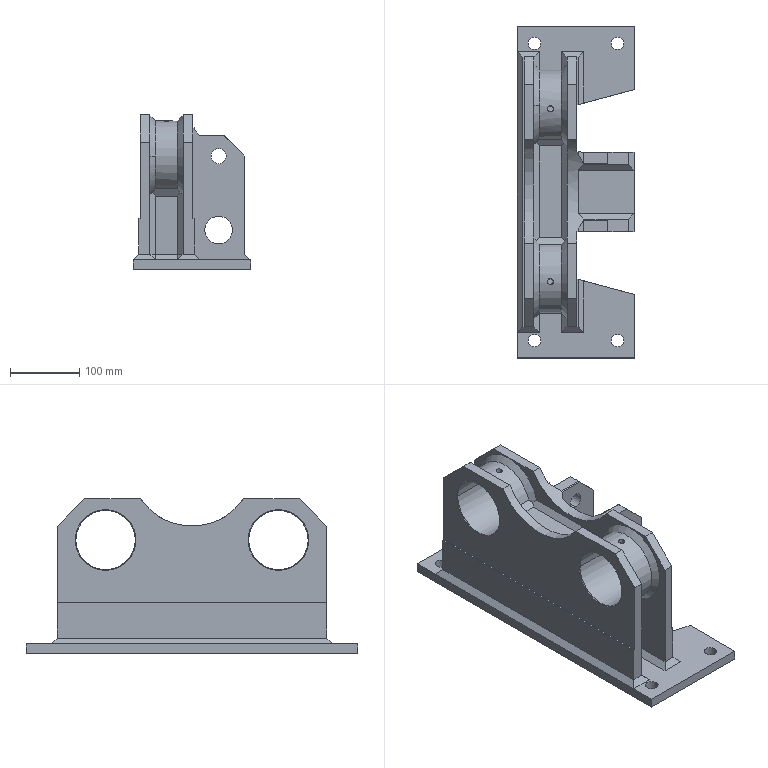Part | SolidWorks | features BaseBody 1 | 1 solid | 146 faces | box 170 x 480 x 224 mm | volume 3738695 mm3 | plane 97 | cylinder 31 | cone 18 | commonest cylinder face diameters 18 x8 101.6 x5 7.95 x4 22 x4 40 x4 86 x4